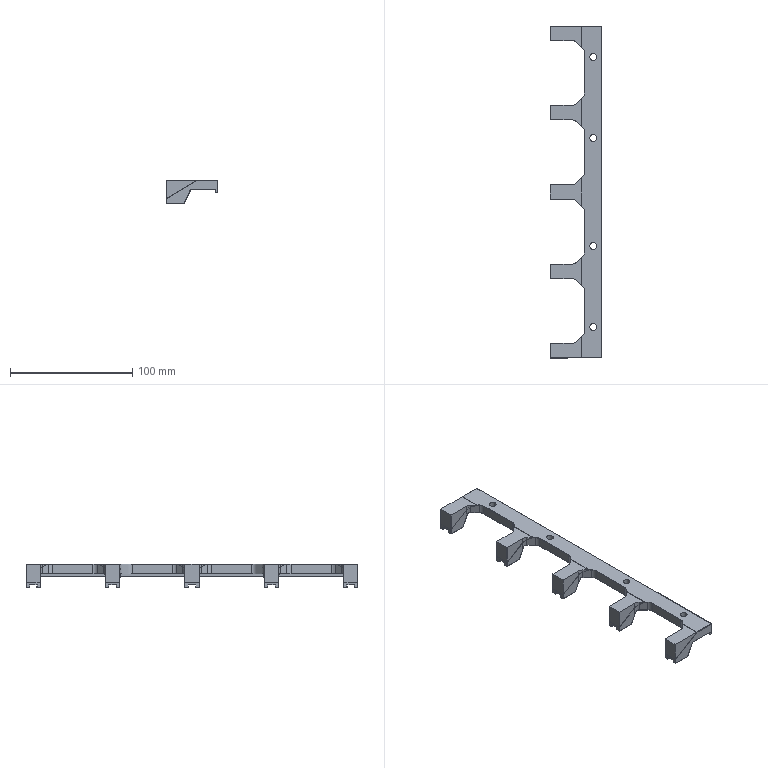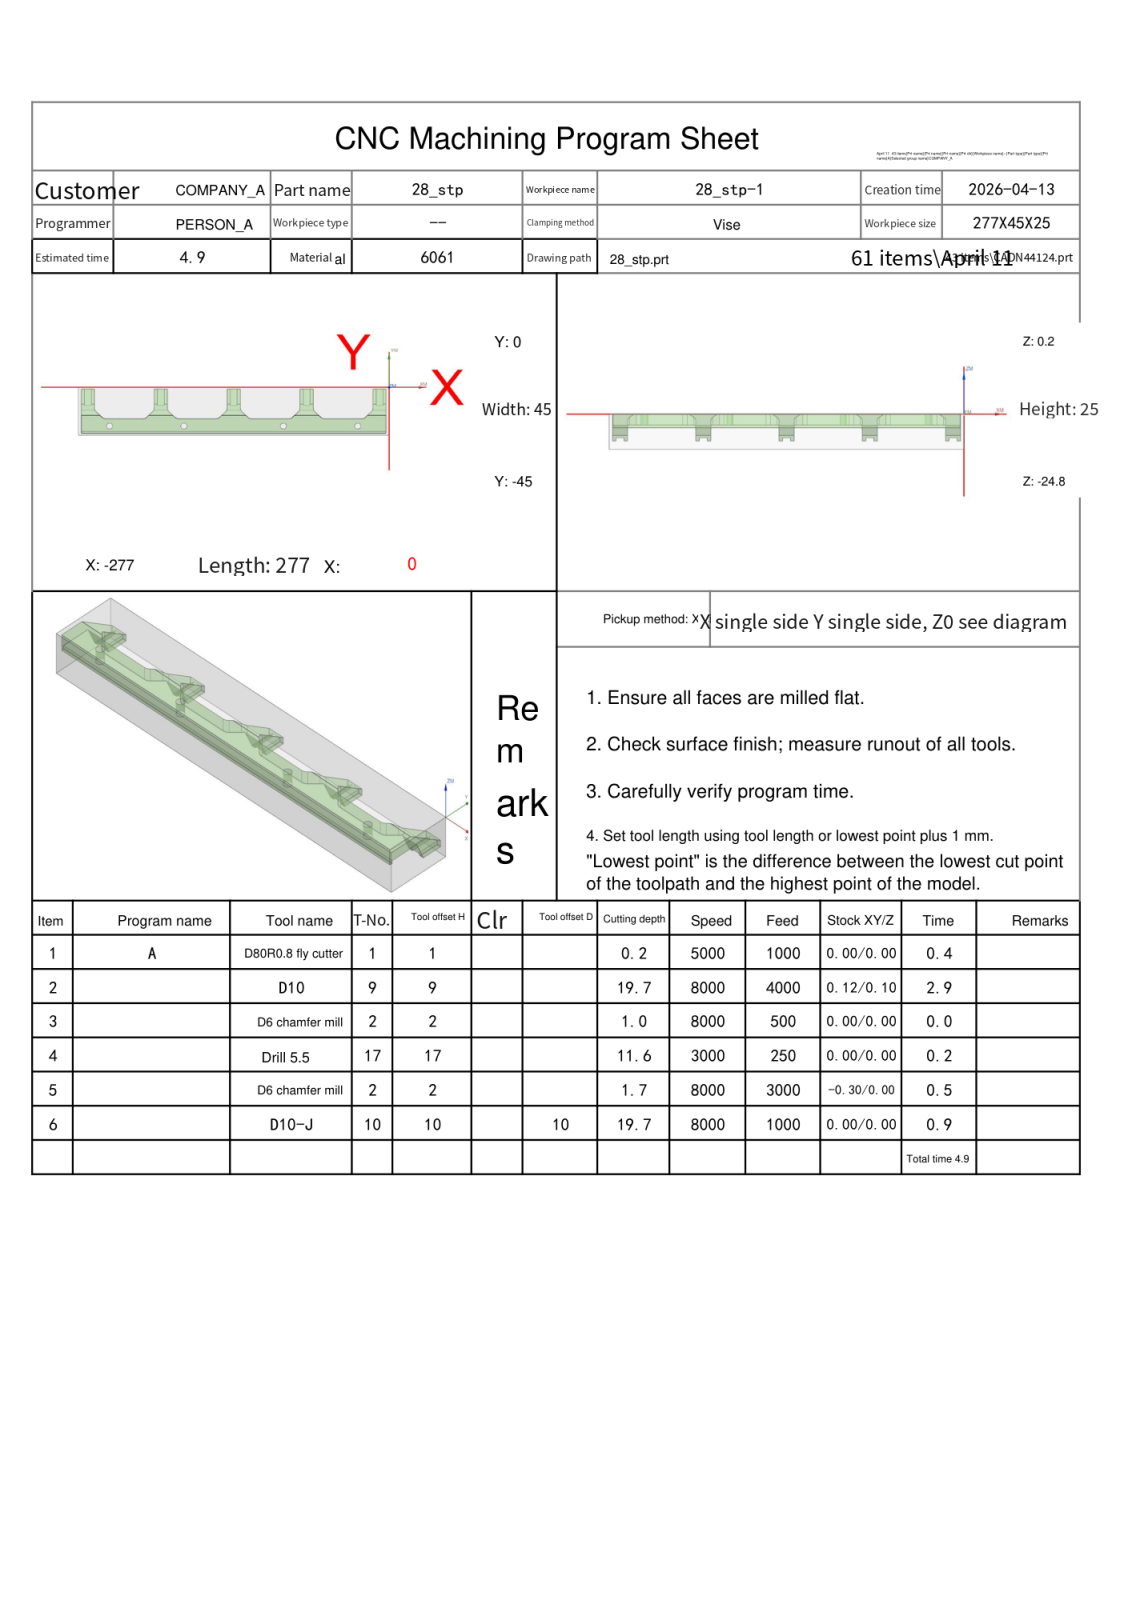NC program | NX | posted by the shop | part box 42 x 271.8 x 19 mm
Lines 32 to 869 of 2830:
N2 T09 M06
(D10  D=10. R=0. H=09 ce=0.12 di=0.10)
G00 G90 G54 X-275.215 Y10.931 M03 S8000
G43 H09 Z20.
M08
Z-17.5
G01 X-275.196 Y10.832 Z-18.125 F4000.
X-275.177 Y10.734 Z-18.372
X-275.159 Y10.636 Z-18.554
X-275.14 Y10.538 Z-18.7
X-275.121 Y10.439 Z-18.823
X-275.103 Y10.341 Z-18.928
X-275.084 Y10.243 Z-19.02
X-275.065 Y10.145 Z-19.1
X-275.047 Y10.046 Z-19.17
X-275.028 Y9.948 Z-19.232
X-275.009 Y9.85 Z-19.286
X-274.991 Y9.752 Z-19.333
X-274.972 Y9.653 Z-19.374
X-274.953 Y9.555 Z-19.408
X-274.935 Y9.457 Z-19.436
X-274.916 Y9.359 Z-19.46
X-274.897 Y9.261 Z-19.477
X-274.879 Y9.162 Z-19.49
X-274.86 Y9.064 Z-19.497
X-274.841 Y8.966 Z-19.5
X-274.44 Y6.852
G03 X-274.181 Y6.5 I.505 J.101
X-270.366 Y5.862 I4.014 J12.275
X-260.196 Y5.681 I10.17 J285.784
X-256.872 Y5.7 I0.0 J285.965
G01 X-1.752 Y5.676
G02 X4.025 Y1.811 I-.242 J-6.612
X5.461 Y-4.139 I-14.623 J-6.679
X5.703 Y-12.252 I-135.848 J-8.113
X5.695 Y-13.734 I-136.09 J0.0
G01 X5.676 Y-43.25
G02 X1.811 Y-49.025 I-6.611 J.244
X-4.139 Y-50.461 I-6.676 J14.611
X-12.252 Y-50.703 I-8.112 J135.793
X-13.734 Y-50.695 I0.0 J136.036
G01 X-275.25 Y-50.676
G02 X-281.025 Y-46.811 I.244 J6.611
X-282.461 Y-40.861 I14.611 J6.676
X-282.703 Y-32.748 I135.794 J8.112
X-282.695 Y-31.266 I136.036 J0.0
G01 X-282.676 Y-1.75
G02 X-278.442 Y4.183 I6.624 J-.25
X-273.754 Y5.018 I4.688 J-12.737
X-273.502 Y5.016 I0.0 J-13.573
G01 X-259.751 Y4.901
X-3.852 Y4.883
G02 X2.658 Y.816 I-.297 J-7.719
X4.502 Y-5.355 I-13.818 J-7.488
X4.901 Y-14.118 I-95.944 J-8.763
X4.89 Y-15.583 I-96.343 J0.0
G01 X4.881 Y-41.167
G02 X.8 Y-47.665 I-7.777 J.354
X-5.37 Y-49.501 I-7.548 J14.082
X-13.11 Y-49.886 I-7.74 J77.583
X-13.997 Y-49.881 I0.0 J77.969
G01 X-273.167
G02 X-279.883 Y-45.504 I.375 J7.916
X-281.558 Y-39.199 I15.573 J7.513
X-281.898 Y-30.644 I107.502 J8.555
X-281.89 Y-29.368 I107.842 J0.0
G01 X-281.881 Y-3.833
G02 X-277.34 Y2.711 I7.377 J-.271
X-272.513 Y3.93 I5.412 J-11.261
X-265.615 Y4.135 I6.898 J-116.048
X-263.158 Y4.109 I0.0 J-116.253
G01 X-5.752 Y4.08
G02 X-3.122 Y3.62 I-.496 J-10.582
G01 X-2.945 Y3.623
G02 X2.317 Y-.257 I0.0 J-5.509
X3.928 Y-9.686 I-31.051 J-10.157
X4.117 Y-21.625 I-376.872 J-11.939
X4.099 Y-25.363 I-377.061 J0.0
X4.115 Y-30.465 I-809.575 J-5.102
X4.064 Y-39.503 I-809.591 J0.0
X2.379 Y-44.184 I-8.571 J.442
G01 X1.876 Y-45.486
G02 X.403 Y-47.26 I-9.155 J6.101
X-3.335 Y-48.64 I-3.738 J4.374
G01 X-3.461 Y-48.638
G02 X-17.355 Y-49.102 I-13.894 J207.761
X-19.295 Y-49.093 I0.0 J208.225
G01 X-271.274 Y-49.077
G02 X-273.901 Y-48.62 I.583 J11.12
X-278.005 Y-46.637 I.07 J5.385
G01 X-278.876 Y-45.486
G02 X-280.831 Y-36.785 I23.796 J9.918
X-281.107 Y-26.786 I181.339 J9.999
X-281.096 Y-24.79 I181.614 J0.0
G01 X-281.08 Y-5.77
G02 X-279.468 Y-1.072 I8.226 J-.196
X-274.2 Y3.62 I5.39 J-.748
G01 X-262.699
G03 X-255.975 Y3.304 I6.724 J71.494
X-254.771 Y3.314 I0.0 J71.809
G01 X-210.98 Y3.312
G02 X-209.307 Y3.62 I1.673 J-4.396
G01 X-209.299
X-197.699
G03 X-190.142 Y3.297 I7.556 J88.366
X-188.699 Y3.309 I0.0 J88.688
G01 X-145.984 Y3.312
G02 X-144.3 Y3.62 I1.684 J-4.447
G01 X-144.299
X-132.699
G03 X-125.105 Y3.297 I7.593 J89.226
X-123.659 Y3.309 I0.0 J89.549
G01 X-80.98 Y3.312
G02 X-79.304 Y3.62 I1.676 J-4.412
G01 X-79.299
X-67.699
G03 X-60.133 Y3.298 I7.565 J88.627
X-58.699 Y3.309 I0.0 J88.95
G01 X-15.942 Y3.317
G02 X-14.299 Y3.62 I1.742 J-4.833
G01 X-3.099
X-14.299
G03 X-16.441 Y3.158 I.23 J-6.263
G02 X-21.319 Y2.71 I-4.878 J26.331
X-21.684 Y2.712 I0.0 J26.779
G01 X-29.751 Y2.661
X-60.894 Y2.69
G02 X-64.981 Y2.83 I1.247 J96.132
G03 X-66.68 Y3.517 I-2.817 J-4.52
G02 X-64.721 Y2.694 I-1.795 J-7.01
G03 X-60.681 Y2.033 I4.327 J13.786
X-50.438 Y1.842 I10.243 J274.016
X-47.192 Y1.861 I0.0 J274.207
G01 X-23.887 Y1.887
G03 X-23.201 Y1.881 I.687 J39.273
X-17.84 Y2.249 I0.0 J39.279
G02 X-16.485 Y3.13 I21.798 J-32.009
G01 X-16.182 Y3.234
G03 X-17.816 Y2.231 I1.902 J-4.929
G02 X-21.08 Y1.484 I-3.673 J8.538
X-29.707 Y1.205 I-8.627 J133.638
X-31.833 Y1.222 I0.0 J133.916
G01 X-55.847 Y1.255
G02 X-56.378 Y1.252 I-.531 J46.069
X-62.866 Y1.711 I0.0 J46.072
X-63.988 Y2.057 I.222 J2.713
G01 X-64.939 Y2.796
G02 X-63.717 Y1.823 I-18.194 J-24.109
G03 X-60.477 Y.862 I4.036 J7.67
X-52.827 Y.442 I7.65 J69.379
X-52.116 Y.446 I0.0 J69.799
G01 X-27.881 Y.444
G03 X-27.12 Y.439 I.761 J52.415
X-20.322 Y.881 I0.0 J52.42
X-18.619 Y1.367 I-.755 J5.869
G01 X-17.717 Y2.309
X-18.631 Y1.325
G02 X-21.513 Y.297 I-3.624 J5.607
X-29.005 Y-.197 I-7.492 J56.525
X-29.795 Y-.192 I0.0 J57.02
G01 X-50.913 Y-.201
G02 X-51.913 Y-.208 I-1. J74.306
X-59.982 Y.232 I0.0 J74.313
X-63.233 Y1.158 I.852 J9.152
G01 X-63.963 Y2.031
G03 X-62.928 Y.842 I6.355 J4.485
X-59.374 Y-.416 I4.594 J7.33
X-51.16 Y-.983 I8.213 J59.201
X-50.578 Y-.98 I0.0 J59.768
X-40.922 Y-1.039 I9.656 J787.989
X-26.943 Y-.915 I0.0 J788.049
X-20.742 Y-.192 I-.142 J28.164
X-19.116 Y.51 I-1.322 J5.292
G02 X-18.575 Y1.387 I14.009 J-8.033
G03 X-19.084 Y.508 I3.197 J-2.435
G02 X-21.52 Y-.756 I-3.467 J3.701
X-28.234 Y-1.545 I-6.937 J30.086
X-40.518 Y-1.68 I-12.285 J558.663
X-53.899 Y-1.52 I0.0 J558.798
X-60.604 Y-.669 I.417 J30.146
X-62.792 Y.348 I1.604 J6.312
G01 X-63.301 Y1.229
G03 X-62.287 Y-.214 I3.85 J1.628
X-58.467 Y-1.702 I5.166 J7.611
X-50.218 Y-2.384 I8.273 J49.861
X-40.717 Y-2.481 I9.501 J466.771
X-28.027 Y-2.308 I0.0 J466.868
X-21.622 Y-1.433 I-.455 J27.184
X-19.47 Y-.358 I-1.544 J5.784
G01 X-19.025 Y.621
G02 X-19.709 Y-.674 I-3.603 J1.072
X-22.903 Y-2.186 I-4.555 J5.495
X-30.07 Y-2.98 I-7.595 J35.813
X-40.304 Y-3.117 I-10.233 J380.375
X-52.808 Y-2.912 I0.0 J380.512
X-59.796 Y-1.9 I.685 J29.371
X-62.528 Y-.412 I1.647 J6.276
X-62.797 Y.324 I7.708 J3.234
G03 X-61.292 Y-1.665 I2.803 J.557
X-56.546 Y-3.218 I6.383 J11.479
X-47.012 Y-3.856 I9.534 J70.899
X-46.531 Y-3.854 I0.0 J71.537
X-40.476 Y-3.912 I6.055 J317.13
X-29.174 Y-3.711 I0.0 J317.188
X-22.388 Y-2.701 I-.689 J27.933
X-19.592 Y-1.083 I-1.507 J5.828
X-19.435 Y-.337 I-2.105 J.832
G01 Y-.34
G02 X-20.359 Y-2.012 I-1.975 J0.0
X-24.607 Y-3.716 I-5.856 J8.451
X-33.37 Y-4.463 I-8.782 J51.237
X-40.206 Y-4.547 I-6.836 J278.253
X-51.816 Y-4.305 I0.0 J278.337
X-59.045 Y-3.176 I.99 J30.046
X-62.185 Y-1.405 I1.996 J7.209
X-62.487 Y-.715 I.64 J.691
G01 X-62.485 Y-.667
X-62.605 Y-.285
G02 X-62.432 Y-1.128 I-3.537 J-1.166
G03 X-60.688 Y-2.932 I3.515 J1.654
X-55.376 Y-4.625 I7.198 J13.403
X-45.291 Y-5.291 I10.085 J76.081
X-44.897 Y-5.29 I0.0 J76.746
X-40.235 Y-5.341 I4.662 J211.638
X-29.555 Y-5.072 I0.0 J211.689
X-22.604 Y-3.833 I-1.022 J25.86
X-19.723 Y-1.972 I-1.98 J6.224
X-19.512 Y-.906 I-3.143 J1.175
G02 X-19.714 Y-2.051 I-3.837 J.085
X-22.064 Y-4.003 I-4.246 J2.721
X-28.179 Y-5.506 I-7.644 J17.909
X-38.678 Y-5.968 I-10.498 J118.977
X-40.546 Y-5.954 I0.0 J119.439
X-42.426 Y-5.968 I-1.881 J123.514
X-53.37 Y-5.482 I0.0 J123.528
X-59.72 Y-3.947 I1.752 J21.155
X-62.317 Y-1.922 I2.237 J5.544
X-62.453 Y-.985 I5.56 J1.287
G01 X-62.454 Y-1.048
G03 X-62.168 Y-2.384 I3.271 J0.0
X-59.336 Y-4.646 I5.083 J3.46
X-52.48 Y-6.278 I8.609 J20.953
X-41.324 Y-6.76 I11.156 J128.708
X-38.975 Y-6.739 I0.0 J129.19
X-37.824 Y-6.746 I1.151 J91.563
X-27.719 Y-6.187 I0.0 J91.57
X-21.774 Y-4.501 I-1.793 J17.648
X-19.659 Y-2.636 I-2.243 J4.676
X-19.614 Y-1.946 I-5.313 J.69
X-19.62 Y-1.698 I-5.358 J0.0
G02 X-19.601 Y-2.052 I-3.343 J-.354
X-19.69 Y-2.82 I-3.362 J0.0
X-21.858 Y-4.939 I-4.298 J2.229
X-27.858 Y-6.745 I-7.933 J15.487
X-38.256 Y-7.372 I-10.398 J85.85
X-39.29 Y-7.366 I0.0 J86.477
X-41.526 Y-7.388 I-2.236 J116.383
X-52.55 Y-6.865 I0.0 J116.405
X-59.367 Y-5.155 I1.955 J22.245
X-62.214 Y-2.869 I2.538 J6.076
G01 X-62.38 Y-2.458
Y-1.738
G03 X-62.404 Y-2.103 I2.788 J-.365
X-61.464 Y-4.201 I2.812 J0.0
X-57.029 Y-6.629 I7.093 J7.694
X-48.23 Y-7.955 I10.039 J36.752
X-40.578 Y-8.174 I7.652 J133.217
X-30.074 Y-7.76 I0.0 J133.436
X-22.929 Y-6.137 I-1.732 J24.162
X-19.805 Y-3.798 I-2.561 J6.677
X-19.62 Y-3.38 I-2.281 J1.258
G01 Y-2.5
G02 X-19.595 Y-2.9 I-3.224 J-.401
X-19.743 Y-3.869 I-3.249 J0.0
X-22.156 Y-6.183 I-4.894 J2.688
X-28.516 Y-8.119 I-8.567 J16.725
X-39.188 Y-8.788 I-10.672 J84.77
X-40.703 Y-8.775 I0.0 J85.44
X-42.011 Y-8.785 I-1.308 J86.45
X-53.057 Y-8.076 I0.0 J86.459
X-59.606 Y-6.099 I2.449 J19.947
X-62.329 Y-3.554 I2.777 J5.701
X-62.4 Y-2.906 I2.91 J.648
X-62.38 Y-2.562 I2.981 J0.0
G03 X-62.404 Y-2.958 I3.311 J-.396
X-62.177 Y-4.164 I3.334 J0.0
X-59.375 Y-6.781 I5.658 J3.251
X-52.456 Y-8.859 I9.412 J18.78
X-41.297 Y-9.566 I11.158 J87.687
X-39.613 Y-9.55 I0.0 J88.394
X-38.671 Y-9.556 I.942 J72.662
X-28.164 Y-8.793 I0.0 J72.668
X-21.935 Y-6.724 I-2.483 J17.886
X-19.645 Y-4.475 I-2.721 J5.063
G01 X-19.62 Y-3.397
G02 X-19.602 Y-3.821 I-5.062 J-.424
X-19.681 Y-4.711 I-5.08 J0.0
X-21.865 Y-7.104 I-4.801 J2.189
X-27.972 Y-9.297 I-8.756 J14.783
X-38.699 Y-10.168 I-10.727 J65.662
X-39.307 Y-10.165 I0.0 J66.532
X-41.286 Y-10.188 I-1.979 J84.549
X-52.406 Y-9.454 I0.0 J84.572
X-59.423 Y-7.293 I2.639 J21.042
X-62.326 Y-4.531 I2.996 J6.056
X-62.396 Y-3.802 I3.759 J.73
X-62.38 Y-3.453 I3.83 J0.0
G03 X-62.403 Y-3.886 I4.025 J-.433
X-62.239 Y-5.028 I4.049 J0.0
X-59.618 Y-7.747 I5.645 J2.817
X-52.808 Y-10.078 I9.706 J17.245
X-41.459 Y-10.952 I11.349 J73.307
X-40.238 Y-10.942 I0.0 J74.18
X-39.099 Y-10.951 I1.139 J67.759
X-28.298 Y-10.085 I0.0 J67.768
X-21.964 Y-7.851 I-2.807 J18.054
X-19.639 Y-5.492 I-2.888 J5.173
G01 X-19.62 Y-4.432
G02 X-19.601 Y-4.864 I-4.848 J-.432
X-19.684 Y-5.764 I-4.868 J0.0
X-21.945 Y-8.277 I-5.045 J2.264
X-28.254 Y-10.618 I-9.234 J15.215
X-39.127 Y-11.558 I-10.873 J62.452
X-39.855 Y-11.553 I0.0 J63.392
X-41.336 Y-11.568 I-1.482 J73.575
X-52.492 Y-10.718 I0.0 J73.59
X-59.445 Y-8.4 I3.053 J20.743
X-62.331 Y-5.561 I3.307 J6.249
X-62.395 Y-4.791 I4.558 J.771
X-62.38 Y-4.413 I4.623 J0.0
G03 X-62.404 Y-4.878 I4.482 J-.464
X-62.247 Y-6.056 I4.506 J0.0
X-59.654 Y-8.851 I5.817 J2.797
X-52.812 Y-11.35 I10.069 J16.949
X-41.392 Y-12.329 I11.42 J66.101
X-40.314 Y-12.321 I0.0 J67.08
X-39.287 Y-12.329 I1.027 J62.41
X-28.352 Y-11.364 I0.0 J62.418
X-21.88 Y-8.929 I-3.089 J18.032
X-19.638 Y-6.566 I-3.097 J5.183
G01 X-19.62 Y-5.429
G02 X-19.601 Y-5.893 I-5.677 J-.464
X-19.679 Y-6.834 I-5.696 J0.0
X-21.962 Y-9.433 I-5.218 J2.281
X-28.528 Y-11.944 I-9.698 J15.518
X-39.525 Y-12.939 I-10.997 J60.285
X-40.541 Y-12.93 I0.0 J61.279
X-41.554 Y-12.939 I-1.013 J63.024
X-53.088 Y-11.874 I0.0 J63.032
X-59.929 Y-9.225 I3.398 J18.93
X-62.352 Y-6.569 I3.515 J5.639
G01 X-62.38 Y-5.479
G03 X-62.405 Y-5.948 I4.434 J-.469
X-62.236 Y-7.163 I4.459 J0.0
X-59.668 Y-9.987 I5.992 J2.869
X-52.848 Y-12.615 I10.39 J16.804
X-41.226 Y-13.704 I11.622 J61.497
X-39.934 Y-13.69 I0.0 J62.585
X-39.246 Y-13.694 I.688 J56.049
X-28.041 Y-12.563 I0.0 J56.053
X-21.583 Y-9.87 I-3.371 J17.173
X-19.64 Y-7.687 I-3.426 J5.005
G01 X-19.62 Y-6.543
G02 X-19.601 Y-7.006 I-5.59 J-.464
X-19.681 Y-7.952 I-5.61 J0.0
X-21.977 Y-10.607 I-5.368 J2.322
X-28.515 Y-13.214 I-9.995 J15.562
X-39.763 Y-14.311 I-11.248 J57.16
X-41.083 Y-14.296 I0.0 J58.256
X-41.66 Y-14.299 I-.577 J56.69
X-53.4 Y-13.07 I0.0 J56.693
X-60.072 Y-10.271 I3.766 J18.328
X-62.361 Y-7.639 I3.666 J5.501
G01 X-62.38 Y-6.58
G03 X-62.402 Y-7.045 I4.849 J-.465
X-62.26 Y-8.213 I4.871 J0.0
X-59.682 Y-11.143 I6.081 J2.752
X-52.77 Y-13.906 I10.737 J16.835
X-41.02 Y-15.07 I11.75 J58.693
X-39.329 Y-15.046 I0.0 J59.857
G01 X-39.147 Y-15.047
G03 X-27.723 Y-13.75 I0.0 J50.971
X-21.405 Y-10.899 I-3.694 J16.61
X-19.642 Y-8.834 I-3.679 J4.925
G01 X-19.62 Y-7.602
G02 X-19.6 Y-8.095 I-6.23 J-.492
X-19.68 Y-9.089 I-6.249 J0.0
X-21.856 Y-11.701 I-5.362 J2.255
X-28.496 Y-14.484 I-10.296 J15.249
X-39.91 Y-15.672 I-11.414 J54.257
X-41.384 Y-15.652 I0.0 J55.445
G01 X-41.681 Y-15.653
G02 X-53.646 Y-14.273 I0.0 J52.559
X-60.258 Y-11.295 I4.035 J17.788
X-62.368 Y-8.734 I3.698 J5.197
G01 X-62.38 Y-7.628
G03 X-62.404 Y-8.13 I5.167 J-.501
X-62.257 Y-9.356 I5.191 J0.0
X-59.598 Y-12.384 I6.299 J2.85
X-52.569 Y-15.228 I11.081 J17.279
X-40.787 Y-16.431 I11.781 J57.124
X-38.261 Y-16.376 I0.0 J58.327
X-27.025 Y-14.817 I-.55 J45.24
X-21.15 Y-11.865 I-4.053 J15.39
X-19.638 Y-9.974 I-3.737 J4.536
G01 X-19.62 Y-8.755
G02 X-19.601 Y-9.247 I-6.475 J-.492
X-19.678 Y-10.24 I-6.494 J0.0
X-21.959 Y-12.97 I-5.557 J2.328
X-28.677 Y-15.804 I-10.609 J15.769
X-40.154 Y-17.028 I-11.477 J53.162
X-42.218 Y-16.989 I0.0 J54.387
X-54.109 Y-15.41 I.331 J48.037
X-60.395 Y-12.365 I4.415 J17.129
X-62.37 Y-9.876 I3.825 J5.062
G01 X-62.38 Y-8.779
G03 X-62.404 Y-9.276 I5.21 J-.498
X-62.253 Y-10.523 I5.234 J0.0
X-59.674 Y-13.526 I6.328 J2.826
X-52.615 Y-16.497 I11.315 J17.014
X-40.716 Y-17.78 I11.899 J54.511
X-37.76 Y-17.702 I0.0 J55.794
X-26.641 Y-15.955 I-.94 J42.24
X-20.956 Y-12.88 I-4.259 J14.666
X-19.626 Y-11.085 I-3.026 J3.633
G01 X-19.62 Y-9.934
G02 X-19.601 Y-10.427 I-6.324 J-.493
X-19.68 Y-11.425 I-6.343 J0.0
X-21.907 Y-14.136 I-5.581 J2.314
X-28.577 Y-17.057 I-10.782 J15.544
X-40.193 Y-18.373 I-11.616 J50.619
X-42.205 Y-18.334 I0.0 J51.934
X-54.292 Y-16.618 I.384 J46.14
X-60.583 Y-13.396 I4.56 J16.656
X-62.363 Y-11.074 I4.086 J4.977
G01 X-62.38 Y-9.94
G03 X-62.404 Y-10.443 I5.234 J-.503
X-62.252 Y-11.7 I5.259 J0.0
X-59.755 Y-14.674 I6.385 J2.827
X-52.44 Y-17.821 I11.631 J16.957
X-40.574 Y-19.124 I11.866 J53.369
X-36.346 Y-18.96 I0.0 J54.673
X-25.824 Y-16.924 I-1.818 J37.598
X-20.553 Y-13.672 I-4.388 J13.012
X-19.62 Y-12.245 I-2.561 J2.692
G01 Y-11.125
G02 X-19.601 Y-11.616 I-6.373 J-.491
X-19.68 Y-12.617 I-6.392 J0.0
X-21.874 Y-15.328 I-5.642 J2.323
X-28.542 Y-18.327 I-10.97 J15.474
X-40.265 Y-19.712 I-11.723 J48.925
X-42.425 Y-19.666 I0.0 J50.31
X-54.55 Y-17.802 I.603 J44.283
X-60.778 Y-14.421 I4.699 J16.082
X-62.38 Y-12.163 I3.495 J4.177
G01 Y-11.123
G03 X-62.403 Y-11.625 I5.56 J-.502
X-62.268 Y-12.845 I5.583 J0.0
X-59.787 Y-15.867 I6.404 J2.729
X-52.618 Y-19.059 I11.727 J16.688
X-40.599 Y-20.46 I12.02 J50.853
X-36.508 Y-20.3 I0.0 J52.254
X-25.774 Y-18.162 I-1.837 J37.234
X-20.556 Y-14.886 I-4.572 J13.075
X-19.62 Y-13.447 I-2.618 J2.727
G01 Y-12.247
G02 X-19.596 Y-12.805 I-6.547 J-.557
X-19.672 Y-13.797 I-6.57 J0.0
X-21.79 Y-16.488 I-5.596 J2.225
X-28.433 Y-19.579 I-11.108 J15.19
X-40.281 Y-21.045 I-11.848 J47.135
X-42.345 Y-21.001 I0.0 J48.601
X-54.46 Y-19.099 I.653 J43.694
X-60.67 Y-15.734 I4.93 J16.51
X-62.38 Y-13.364 I3.584 J4.389
G01 Y-12.244
G03 X-62.404 Y-12.781 I5.912 J-.537
X-62.267 Y-14.05 I5.936 J0.0
X-59.768 Y-17.108 I6.501 J2.762
X-52.661 Y-20.332 I11.861 J16.702
X-40.572 Y-21.791 I12.089 J49.345
X-35.997 Y-21.585 I0.0 J50.804
X-25.439 Y-19.287 I-2.212 J35.573
X-20.461 Y-16.001 I-4.741 J12.595
X-19.62 Y-14.655 I-2.493 J2.494
G01 Y-13.455
G02 X-19.596 Y-14.017 I-6.581 J-.561
X-19.671 Y-15.012 I-6.605 J0.0
X-21.904 Y-17.813 I-5.775 J2.313
X-28.803 Y-20.962 I-11.437 J15.922
X-40.498 Y-22.377 I-11.695 J47.616
X-44.277 Y-22.232 I0.0 J49.031
X-55.639 Y-19.94 I1.849 J38.476
X-61.16 Y-16.47 I5.108 J14.255
X-62.38 Y-14.573 I3.518 J3.604
G01 Y-13.453
G03 X-62.405 Y-13.991 I5.87 J-.538
X-62.264 Y-15.269 I5.894 J0.0
X-59.702 Y-18.395 I6.602 J2.798
X-52.359 Y-21.698 I12.141 J17.179
X-40.581 Y-23.115 I11.778 J48.249
X-29.095 Y-21.768 I0.0 J49.666
X-21.906 Y-18.566 I-4.596 J19.985
X-19.641 Y-15.992 I-4.156 J5.941
G01 X-19.62 Y-14.685
G02 X-19.601 Y-15.21 I-7.147 J-.525
X-19.677 Y-16.257 I-7.166 J0.0
X-21.834 Y-19. I-5.751 J2.301
X-28.687 Y-22.216 I-11.526 J15.652
X-40.313 Y-23.682 I-11.626 J45.354
X-43.117 Y-23.598 I0.0 J46.82
X-55.28 Y-21.347 I.961 J39.185
X-61.023 Y-17.846 I5.236 J15.05
X-62.38 Y-15.792 I3.728 J3.939
G01 Y-14.672
G03 X-62.405 Y-15.212 I5.862 J-.54
X-62.263 Y-16.498 I5.887 J0.0
X-59.794 Y-19.568 I6.601 J2.781
X-52.607 Y-22.918 I12.158 J16.696
X-41.852 Y-24.38 I11.441 J43.87
X-40.328 Y-24.404 I1.524 J47.511
X-29.445 Y-23.142 I0.0 J47.535
X-22.067 Y-19.933 I-4.622 J20.71
X-19.641 Y-17.225 I-4.213 J6.217
G01 X-19.62 Y-15.919
G02 X-19.603 Y-16.435 I-7.806 J-.516
X-19.673 Y-17.479 I-7.823 J0.0
X-21.825 Y-20.241 I-5.782 J2.285
X-28.713 Y-23.506 I-11.641 J15.662
X-32.692 Y-24.38 I-11.716 J43.829
G01 X-38.772
G03 X-35.552 Y-24.401 I3.219 J241.504
X-30.336 Y-24.345 I0.0 J241.525
X-21.319 Y-20.572 I-1.874 J17.138
X-19.628 Y-18.405 I-3.643 J4.587
G01 X-19.62 Y-17.161
G02 X-19.6 Y-17.688 I-7.071 J-.526
X-19.678 Y-18.735 I-7.091 J0.0
X-21.821 Y-21.48 I-5.77 J2.297
X-27.853 Y-24.38 I-9.962 J12.999
G01 X-30.893
G03 X-29.906 Y-24.383 I.987 J145.692
X-26.784 Y-24.35 I0.0 J145.696
X-23.455 Y-23.214 I-1.52 J9.906
G01 X-19.827 Y-19.555
G03 X-19.62 Y-19.063 I-.968 J.696
G01 Y-18.423
G02 X-19.595 Y-18.74 I-2.032 J-.318
X-19.73 Y-19.474 I-2.057 J0.0
G01 X-23.781 Y-23.519
G02 X-25.453 Y-24.38 I-3.306 J4.364
G01 X-27.133
X-24.947 Y-24.353
G03 X-24.382 Y-24.141 I-.286 J1.617
G01 X-23.59 Y-23.349
X-24.549 Y-24.284
G02 X-25.056 Y-24.388 I-.507 J1.19
G01 X-25.197 Y-24.38
G02 X-25.582 Y-24.199 I.005 J.511
G01 X-26.215 Y-23.435
X-27.473 Y-21.917 Z-19.4
X-27.557 Y-21.816
X-27.607 Y-21.763
X-27.665 Y-21.719
X-27.729 Y-21.683
X-27.797 Y-21.656
X-27.869 Y-21.64
X-27.942 Y-21.635
X-39.107
X-39.18 Y-21.64
X-39.251 Y-21.656
X-39.32 Y-21.683
X-39.383 Y-21.719
X-39.441 Y-21.763
X-39.492 Y-21.816
X-39.561 Y-21.9
X-40.819 Y-23.418 Z-19.5
X-41.517 Y-24.252
G02 X-41.852 Y-24.38 I-.344 J.398
X-43.986 Y-24.405 I-2.135 J91.266
X-48.104 Y-24.312 I0.0 J91.291
X-58.609 Y-20.988 I2.242 J25.344
X-62.162 Y-17.558 I4.837 J8.566
G01 X-62.38 Y-17.017
Y-15.897
G03 X-62.404 Y-16.434 I5.968 J-.536
X-62.262 Y-17.732 I5.992 J0.0
X-59.726 Y-20.871 I6.692 J2.812
X-51.787 Y-24.38 I12.321 J17.14
G01 X-46.907
X-47.386
G02 X-52.829 Y-24.352 I0.0 J526.454
X-61.287 Y-20.036 I2.01 J14.386
X-62.38 Y-18.259 I3.602 J3.44
G01 Y-17.139
G03 X-62.405 Y-17.679 I5.917 J-.54
X-62.262 Y-18.971 I5.942 J0.0
X-61.729 Y-20.031 I6.809 J2.767
X-59.104 Y-22.489 I17.083 J15.613
X-55.306 Y-24.38 I8.002 J11.309
G01 X-52.426
G02 X-53.676 Y-24.399 I-1.25 J42.073
X-55.941 Y-24.338 I0.0 J42.091
X-58.294 Y-23.465 I1.485 J7.612
G01 X-59.991 Y-21.768
G03 X-57.719 Y-23.981 I22.161 J20.479
X-56.922 Y-24.38 I1.558 J2.119
G01 X-55.482
G02 X-56.13 Y-24.4 I-.648 J10.328
X-57.277 Y-24.337 I0.0 J10.348
X-58.054 Y-23.705 I.886 J1.885
G03 X-57.234 Y-24.369 I1.657 J1.209
G01 X-57.043 Y-24.38
X-57.097 Y-24.382
G02 X-57.56 Y-24.199 I0.0 J.676
X-62.139 Y-19.581 I141.995 J145.371
X-62.38 Y-19.05 I1.316 J.917
G01 Y-18.41
G03 X-62.403 Y-18.729 I2.241 J-.319
X-62.284 Y-19.451 I2.263 J0.0
G01 X-61.973 Y-19.787
G03 X-61.616 Y-19.93 I.357 J.371
X-61.173 Y-19.677 I0.0 J.515
G01 X-59.922 Y-18.153 Z-19.4
X-58.949 Y-16.967
X-58.901 Y-16.896
X-58.865 Y-16.818
X-58.843 Y-16.735
X-58.836 Y-16.65
Y-5.531
X-58.843 Y-4.971
X-58.863 Y-4.412
X-58.898 Y-3.853
X-58.946 Y-3.296
X-59.009 Y-2.74
X-59.085 Y-2.186
X-59.174 Y-1.633
X-59.277 Y-1.083
X-59.394 Y-.536
X-59.525 Y.008
X-59.668 Y.549
X-59.826 Y1.086
X-59.996 Y1.619
X-60.947 Y4.473
X-61.008 Y4.631
X-61.081 Y4.783
X-61.168 Y4.928
X-61.267 Y5.066
X-61.377 Y5.194
X-61.498 Y5.312
X-61.628 Y5.419
X-61.768 Y5.515
X-61.915 Y5.599
X-62.069 Y5.669
X-62.228 Y5.726
X-62.392 Y5.769
X-63.709 Y6.054
X-64.311 Y6.178
X-64.916 Y6.289
X-65.522 Y6.388
X-66.131 Y6.474
X-66.742 Y6.547
X-67.353 Y6.607
X-67.966 Y6.654
X-68.58 Y6.689
X-78.762 Y7.154
X-78.848 Y7.151
X-78.932 Y7.133
X-79.011 Y7.101
X-79.084 Y7.055
X-79.148 Y6.998
X-79.202 Y6.931
X-79.243 Y6.855
X-79.575 Y6.095
X-80.364 Y4.289 Z-19.5
X-80.711 Y3.515
G02 X-81.489 Y3.16 I-.927 J1.004
X-86.36 Y2.71 I-4.871 J26.147
X-86.725 Y2.713 I0.0 J26.597
G01 X-94.791 Y2.661
X-125.934 Y2.691
X-129.931 Y2.815
G03 X-131.683 Y3.518 I-3.234 J-5.526
G02 X-129.653 Y2.663 I-2.056 J-7.724
G03 X-125.205 Y2.007 I4.61 J15.841
X-116.544 Y1.86 I8.662 J255.123
X-115.511 Y1.862 I0.0 J255.27
G01 X-88.928 Y1.888
G03 X-88.318 Y1.883 I.609 J40.926
X-82.834 Y2.252 I0.0 J40.931
X-82.195 Y2.723 I-2.899 J4.609
G01 X-81.296 Y3.215
G03 X-82.808 Y2.233 I2.384 J-5.327
G02 X-86.117 Y1.483 I-3.734 J8.801
X-94.175 Y1.215 I-8.058 J120.812
X-95.757 Y1.225 I0.0 J121.08
G01 X-120.495 Y1.251
G02 X-121.122 Y1.247 I-.628 J49.798
X-127.776 Y1.693 I0.0 J49.802
X-128.985 Y2.056 I.189 J2.827
G01 X-129.885 Y2.768
G03 X-128.538 Y1.715 I12.884 J15.09
X-124.568 Y.75 I4.604 J10.297
X-116.292 Y.426 I8.277 J105.476
X-115.176 Y.432 I0.0 J105.8
G01 X-92.684 Y.447
G03 X-91.948 Y.442 I.737 J49.065
X-85.159 Y.914 I0.0 J49.07
X-83.611 Y1.363 I-1.118 J6.745
G02 X-82.706 Y2.307 I4.464 J-3.373
G03 X-83.647 Y1.306 I3.296 J-4.04
G02 X-86.543 Y.294 I-3.671 J5.854
X-93.883 Y-.191 I-7.34 J55.286
X-94.521 Y-.188 I0.0 J55.771
G01 X-115.161 Y-.206
G02 X-116.391 Y-.215 I-1.231 J84.435
X-124.742 Y.199 I0.0 J84.444
X-128.185 Y1.119 I1.004 J10.649
G01 X-128.967 Y2.034
G03 X-127.942 Y.85 I6.681 J4.751
X-124.47 Y-.398 I4.535 J7.155
X-116.594 Y-.969 I7.877 J54.062
G01 X-116.323
G03 X-105.883 Y-1.039 I10.439 J774.336
X-91.905 Y-.913 I0.0 J774.406
X-85.648 Y-.165 I-.118 J27.534
X-84.125 Y.502 I-1.309 J5.057
G01 X-83.59 Y1.362
X-84.146 Y.446
G02 X-86.832 Y-.836 I-3.71 J4.32
X-93.884 Y-1.566 I-7.137 J34.529
X-105.337 Y-1.681 I-11.452 J572.062
X-118.897 Y-1.52 I0.0 J572.177
X-125.636 Y-.661 I.406 J30.033
X-127.825 Y.386 I1.286 J5.503
G01 X-128.274 Y1.179
G03 X-127.218 Y-.27 I3.569 J1.49
X-123.372 Y-1.722 I5.226 J8.024
X-114.877 Y-2.396 I8.495 J53.203
G01 X-114.711
G03 X-105.779 Y-2.482 I8.932 J463.664
X-92.989 Y-2.305 I0.0 J463.75
X-86.592 Y-1.42 I-.454 J26.849
X-84.446 Y-.325 I-1.422 J5.436
G01 X-84.084 Y.538
G03 X-84.418 Y-.332 I5.127 J-2.469
G02 X-86.6 Y-1.781 I-3.487 J2.884
X-92.481 Y-2.839 I-6.768 J20.74
X-102.983 Y-3.112 I-10.503 J201.88
X-105.507 Y-3.097 I0.0 J202.153
X-108.264 Y-3.115 I-2.757 J202.362
X-119.376 Y-2.81 I0.0 J202.381
X-125.58 Y-1.624 I.984 J21.958
X-127.569 Y-.35 I1.625 J4.726
G01 X-127.798 Y.327
G03 X-126.271 Y-1.68 I2.828 J.568
X-121.446 Y-3.235 I6.424 J11.667
X-111.982 Y-3.856 I9.464 J71.898
X-111.57 Y-3.854 I0.0 J72.518
X-105.46 Y-3.917 I6.11 J298.403
X-93.834 Y-3.69 I0.0 J298.466
X-87.292 Y-2.669 I-.815 J26.677
X-84.633 Y-1.142 I-1.629 J5.916
X-84.37 Y-.207 I-15.598 J4.893
X-84.564 Y-1.069 I3.823 J-1.316
G02 X-86.509 Y-2.723 I-3.437 J2.07
X-92.24 Y-4.115 I-6.997 J16.321
X-102.666 Y-4.542 I-10.426 J126.872
X-104.538 Y-4.529 I0.0 J127.3
X-107.19 Y-4.549 I-2.652 J175.535
X-118.356 Y-4.193 I0.0 J175.555
X-124.901 Y-2.864 I1.254 J22.949
X-127.402 Y-1.126 I1.846 J5.326
G01 X-127.606 Y-.284
G02 X-127.434 Y-1.124 I-3.407 J-1.135
G03 X-125.665 Y-2.947 I3.513 J1.64
X-120.195 Y-4.654 I7.276 J13.694
X-109.92 Y-5.301 I10.275 J81.34
X-109.307 Y-5.299 I0.0 J81.986
X-105.045 Y-5.345 I4.262 J195.379
X-94.143 Y-5.041 I0.0 J195.426
X-87.508 Y-3.796 I-1.172 J24.554
X-84.712 Y-1.944 I-1.928 J5.947
X-84.545 Y-1.066 I-2.23 J.878
G01 X-84.547 Y-.982
X-84.546 Y-1.065
G02 X-84.721 Y-2.056 I-2.889 J0.0
X-87.039 Y-3.99 I-4.212 J2.692
X-93.216 Y-5.509 I-7.673 J17.877
X-103.574 Y-5.966 I-10.358 J117.223
X-105.27 Y-5.954 I0.0 J117.679
X-107.182 Y-5.968 I-1.912 J131.903
X-117.998 Y-5.524 I0.0 J131.917
X-124.576 Y-4.014 I1.657 J22.306
X-127.313 Y-1.928 I2.177 J5.694
X-127.453 Y-.985 I4.688 J1.179
G01 X-127.454 Y-1.045
G03 X-127.167 Y-2.386 I3.282 J0.0
X-124.309 Y-4.659 I5.113 J3.496
X-117.589 Y-6.266 I8.536 J20.837
X-106.363 Y-6.761 I11.226 J127.029
X-104.014 Y-6.74 I0.0 J127.524
X-102.836 Y-6.747 I1.179 J91.3
X-92.683 Y-6.181 I0.0 J91.308
X-86.713 Y-4.467 I-1.782 J17.457
X-84.643 Y-2.577 I-2.014 J4.286
G01 X-84.62 Y-1.699
G02 X-84.595 Y-2.078 I-2.883 J-.38
X-84.69 Y-2.815 I-2.908 J0.0
X-86.883 Y-4.951 I-4.325 J2.245
X-92.824 Y-6.739 I-7.912 J15.527
X-103.163 Y-7.37 I-10.339 J84.337
X-104.095 Y-7.365 I0.0 J84.968
X-106.434 Y-7.388 I-2.339 J118.903
X-117.439 Y-6.878 I0.0 J118.926
X-124.209 Y-5.229 I1.993 J22.9
X-127.231 Y-2.84 I2.455 J6.212
G01 X-127.38 Y-2.463
Y-1.743
G03 X-127.404 Y-2.109 I2.792 J-.366
X-126.412 Y-4.254 I2.816 J0.0
X-121.934 Y-6.658 I7.151 J7.947
X-113.192 Y-7.958 I10.004 J37.248
X-105.587 Y-8.176 I7.605 J132.342
X-95.036 Y-7.755 I0.0 J132.561
X-87.982 Y-6.159 I-1.785 J24.276
X-84.828 Y-3.829 I-2.596 J6.815
X-84.62 Y-3.369 I-1.533 J.97
G01 Y-2.489
G02 X-84.602 Y-2.884 I-4.41 J-.395
X-84.682 Y-3.722 I-4.428 J0.0
X-86.886 Y-6.021 I-4.586 J2.189
X-92.851 Y-8.01 I-8.311 J14.986
X-103.394 Y-8.773 I-10.543 J72.474
X-104.104 Y-8.77 I0.0 J73.237
X-106.328 Y-8.795 I-2.224 J98.626
X-117.438 Y-8.167 I0.0 J98.651
X-124.257 Y-6.284 I2.362 J21.845